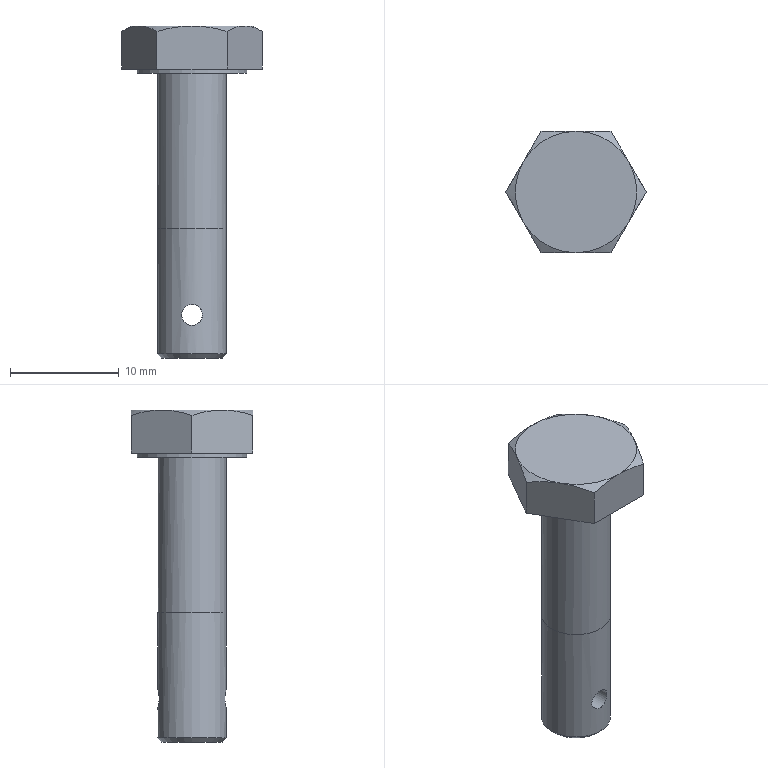Part | NX | features solid 2 | 1 solid | 21 faces | box 12.905 x 11.176 x 30.563 mm | volume 1269 mm3 | plane 10 | cone 7 | cylinder 4 | commonest cylinder face diameters 6.35 x2 1.93 x1 10.109 x1
STEP:
#1=CARTESIAN_POINT('',(0.,-3.175,-27.559));
#2=VERTEX_POINT('',#1);
#3=CARTESIAN_POINT('',(0.7569,-3.102,-27.35));
#4=CARTESIAN_POINT('',(-0.00006064,-3.212,-27.664));
#5=CARTESIAN_POINT('',(-0.7566,-3.102,-27.349));
#6=CARTESIAN_POINT('',(-1.07,-2.986,-26.595));
#7=CARTESIAN_POINT('',(-0.7562,-3.102,-25.837));
#8=CARTESIAN_POINT('',(-0.0005897,-3.212,-25.524));
#9=CARTESIAN_POINT('',(0.7561,-3.102,-25.837));
#10=CARTESIAN_POINT('',(1.07,-2.986,-26.594));
#11=CARTESIAN_POINT('',(0.7569,-3.102,-27.35));
#12=CARTESIAN_POINT('',(-0.00006064,-3.212,-27.664));
#13=CARTESIAN_POINT('',(-0.7566,-3.102,-27.349));
#14=B_SPLINE_CURVE_WITH_KNOTS('',3,(#3,#4,#5,#6,#7,#8,#9,#10,#11,#12,#13),.UNSPECIFIED.,.T.,.F.,(1,1,1,1,1,1,1,1,1,1,1,1,1,1,1),(-0.002276,-0.001518,-0.0007588,0.,0.0007588,0.001518,0.002276,0.003035,0.003794,0.004553,0.005312,0.006071,0.006829,0.007588,0.008347),.UNSPECIFIED.);
#15=EDGE_CURVE('',#2,#2,#14,.T.);
#16=ORIENTED_EDGE('',*,*,#15,.T.);
#17=EDGE_LOOP('',(#16));
#18=FACE_BOUND('',#17,.T.);
#19=CARTESIAN_POINT('',(-3.175,0.,-18.656));
#20=VERTEX_POINT('',#19);
#21=CARTESIAN_POINT('',(-2.488,2.488,-18.656));
#22=CARTESIAN_POINT('',(-3.519,0.,-18.656));
#23=CARTESIAN_POINT('',(-2.488,-2.488,-18.656));
#24=CARTESIAN_POINT('',(0.,-3.519,-18.656));
#25=CARTESIAN_POINT('',(2.488,-2.488,-18.656));
#26=CARTESIAN_POINT('',(3.519,0.,-18.656));
#27=CARTESIAN_POINT('',(2.488,2.488,-18.656));
#28=CARTESIAN_POINT('',(0.,3.519,-18.656));
#29=CARTESIAN_POINT('',(-2.488,2.488,-18.656));
#30=CARTESIAN_POINT('',(-3.519,0.,-18.656));
#31=CARTESIAN_POINT('',(-2.488,-2.488,-18.656));
#32=B_SPLINE_CURVE_WITH_KNOTS('',3,(#21,#22,#23,#24,#25,#26,#27,#28,#29,#30,#31),.UNSPECIFIED.,.T.,.F.,(1,1,1,1,1,1,1,1,1,1,1,1,1,1,1),(-0.375,-0.25,-0.125,0.,0.125,0.25,0.375,0.5,0.625,0.75,0.875,1.,1.125,1.25,1.375),.UNSPECIFIED.);
#33=EDGE_CURVE('',#20,#20,#32,.T.);
#34=ORIENTED_EDGE('',*,*,#33,.F.);
#35=EDGE_LOOP('',(#34));
#36=FACE_BOUND('',#35,.T.);
#37=CARTESIAN_POINT('',(-3.175,0.,-30.182));
#38=VERTEX_POINT('',#37);
#39=CARTESIAN_POINT('',(0.,0.,-30.182));
#40=DIRECTION('',(0.,0.,-1.));
#41=DIRECTION('',(-1.,0.,0.));
#42=AXIS2_PLACEMENT_3D('',#39,#40,#41);
#43=CIRCLE('',#42,3.175);
#44=EDGE_CURVE('',#38,#38,#43,.T.);
#45=ORIENTED_EDGE('',*,*,#44,.F.);
#46=EDGE_LOOP('',(#45));
#47=FACE_BOUND('',#46,.T.);
#48=CARTESIAN_POINT('',(0.,3.175,-27.559));
#49=VERTEX_POINT('',#48);
#50=CARTESIAN_POINT('',(-0.7569,3.102,-27.35));
#51=CARTESIAN_POINT('',(0.00006064,3.212,-27.664));
#52=CARTESIAN_POINT('',(0.7566,3.102,-27.349));
#53=CARTESIAN_POINT('',(1.07,2.986,-26.595));
#54=CARTESIAN_POINT('',(0.7562,3.102,-25.837));
#55=CARTESIAN_POINT('',(0.0005897,3.212,-25.524));
#56=CARTESIAN_POINT('',(-0.7561,3.102,-25.837));
#57=CARTESIAN_POINT('',(-1.07,2.986,-26.594));
#58=CARTESIAN_POINT('',(-0.7569,3.102,-27.35));
#59=CARTESIAN_POINT('',(0.00006064,3.212,-27.664));
#60=CARTESIAN_POINT('',(0.7566,3.102,-27.349));
#61=B_SPLINE_CURVE_WITH_KNOTS('',3,(#50,#51,#52,#53,#54,#55,#56,#57,#58,#59,#60),.UNSPECIFIED.,.T.,.F.,(1,1,1,1,1,1,1,1,1,1,1,1,1,1,1),(-0.002276,-0.001518,-0.0007588,0.,0.0007588,0.001518,0.002276,0.003035,0.003794,0.004553,0.005312,0.006071,0.006829,0.007588,0.008347),.UNSPECIFIED.);
#62=EDGE_CURVE('',#49,#49,#61,.T.);
#63=ORIENTED_EDGE('',*,*,#62,.T.);
#64=EDGE_LOOP('',(#63));
#65=FACE_BOUND('',#64,.T.);
#66=CARTESIAN_POINT('',(0.,0.,0.));
#67=DIRECTION('',(0.,0.,-1.));
#68=DIRECTION('',(-1.,0.,0.));
#69=AXIS2_PLACEMENT_3D('',#66,#67,#68);
#70=CYLINDRICAL_SURFACE('',#69,3.175);
#71=ADVANCED_FACE('',(#18,#36,#47,#65),#70,.T.);
#72=CARTESIAN_POINT('',(-3.175,0.,-4.369));
#73=VERTEX_POINT('',#72);
#74=CARTESIAN_POINT('',(0.,0.,-4.369));
#75=DIRECTION('',(0.,0.,-1.));
#76=DIRECTION('',(-1.,0.,0.));
#77=AXIS2_PLACEMENT_3D('',#74,#75,#76);
#78=CIRCLE('',#77,3.175);
#79=EDGE_CURVE('',#73,#73,#78,.T.);
#80=ORIENTED_EDGE('',*,*,#79,.T.);
#81=EDGE_LOOP('',(#80));
#82=FACE_BOUND('',#81,.T.);
#83=ORIENTED_EDGE('',*,*,#33,.T.);
#84=EDGE_LOOP('',(#83));
#85=FACE_BOUND('',#84,.T.);
#86=CARTESIAN_POINT('',(0.,0.,0.));
#87=DIRECTION('',(0.,0.,-1.));
#88=DIRECTION('',(-1.,0.,0.));
#89=AXIS2_PLACEMENT_3D('',#86,#87,#88);
#90=CYLINDRICAL_SURFACE('',#89,3.175);
#91=ADVANCED_FACE('',(#82,#85),#90,.T.);
#92=CARTESIAN_POINT('',(-6.452,0.,-3.962));
#93=VERTEX_POINT('',#92);
#94=CARTESIAN_POINT('',(-3.226,5.588,-3.962));
#95=VERTEX_POINT('',#94);
#96=CARTESIAN_POINT('',(-3.576,4.983,-3.962));
#97=DIRECTION('',(0.5,0.866,0.));
#98=VECTOR('',#97,1000.);
#99=LINE('',#96,#98);
#100=EDGE_CURVE('',#93,#95,#99,.T.);
#101=ORIENTED_EDGE('',*,*,#100,.T.);
#102=CARTESIAN_POINT('',(3.226,5.588,-3.962));
#103=VERTEX_POINT('',#102);
#104=CARTESIAN_POINT('',(5.055,5.588,-3.962));
#105=DIRECTION('',(1.,0.,0.));
#106=VECTOR('',#105,1000.);
#107=LINE('',#104,#106);
#108=EDGE_CURVE('',#95,#103,#107,.T.);
#109=ORIENTED_EDGE('',*,*,#108,.T.);
#110=CARTESIAN_POINT('',(6.452,0.,-3.962));
#111=VERTEX_POINT('',#110);
#112=CARTESIAN_POINT('',(6.103,0.6053,-3.962));
#113=DIRECTION('',(0.5,-0.866,0.));
#114=VECTOR('',#113,1000.);
#115=LINE('',#112,#114);
#116=EDGE_CURVE('',#103,#111,#115,.T.);
#117=ORIENTED_EDGE('',*,*,#116,.T.);
#118=CARTESIAN_POINT('',(3.226,-5.588,-3.962));
#119=VERTEX_POINT('',#118);
#120=CARTESIAN_POINT('',(6.103,-0.6053,-3.962));
#121=DIRECTION('',(-0.5,-0.866,0.));
#122=VECTOR('',#121,1000.);
#123=LINE('',#120,#122);
#124=EDGE_CURVE('',#111,#119,#123,.T.);
#125=ORIENTED_EDGE('',*,*,#124,.T.);
#126=CARTESIAN_POINT('',(-3.226,-5.588,-3.962));
#127=VERTEX_POINT('',#126);
#128=CARTESIAN_POINT('',(5.055,-5.588,-3.962));
#129=DIRECTION('',(-1.,0.,0.));
#130=VECTOR('',#129,1000.);
#131=LINE('',#128,#130);
#132=EDGE_CURVE('',#119,#127,#131,.T.);
#133=ORIENTED_EDGE('',*,*,#132,.T.);
#134=CARTESIAN_POINT('',(-3.576,-4.983,-3.962));
#135=DIRECTION('',(-0.5,0.866,0.));
#136=VECTOR('',#135,1000.);
#137=LINE('',#134,#136);
#138=EDGE_CURVE('',#127,#93,#137,.T.);
#139=ORIENTED_EDGE('',*,*,#138,.T.);
#140=EDGE_LOOP('',(#101,#109,#117,#125,#133,#139));
#141=FACE_BOUND('',#140,.T.);
#142=CARTESIAN_POINT('',(-5.055,0.,-3.962));
#143=VERTEX_POINT('',#142);
#144=CARTESIAN_POINT('',(0.,0.,-3.962));
#145=DIRECTION('',(0.,0.,-1.));
#146=DIRECTION('',(-1.,0.,0.));
#147=AXIS2_PLACEMENT_3D('',#144,#145,#146);
#148=CIRCLE('',#147,5.055);
#149=EDGE_CURVE('',#143,#143,#148,.T.);
#150=ORIENTED_EDGE('',*,*,#149,.F.);
#151=EDGE_LOOP('',(#150));
#152=FACE_BOUND('',#151,.T.);
#153=CARTESIAN_POINT('',(5.055,0.,-3.962));
#154=DIRECTION('',(0.,0.,-1.));
#155=DIRECTION('',(-1.,0.,0.));
#156=AXIS2_PLACEMENT_3D('',#153,#154,#155);
#157=PLANE('',#156);
#158=ADVANCED_FACE('',(#141,#152),#157,.T.);
#159=CARTESIAN_POINT('',(-2.794,0.,-30.563));
#160=VERTEX_POINT('',#159);
#161=CARTESIAN_POINT('',(0.,0.,-30.563));
#162=DIRECTION('',(0.,0.,-1.));
#163=DIRECTION('',(-1.,0.,0.));
#164=AXIS2_PLACEMENT_3D('',#161,#162,#163);
#165=CIRCLE('',#164,2.794);
#166=EDGE_CURVE('',#160,#160,#165,.T.);
#167=ORIENTED_EDGE('',*,*,#166,.T.);
#168=EDGE_LOOP('',(#167));
#169=FACE_BOUND('',#168,.T.);
#170=CARTESIAN_POINT('',(0.,0.,-30.563));
#171=DIRECTION('',(0.,0.,-1.));
#172=DIRECTION('',(-1.,0.,0.));
#173=AXIS2_PLACEMENT_3D('',#170,#171,#172);
#174=PLANE('',#173);
#175=ADVANCED_FACE('',(#169),#174,.T.);
#176=ORIENTED_EDGE('',*,*,#44,.T.);
#177=EDGE_LOOP('',(#176));
#178=FACE_BOUND('',#177,.T.);
#179=ORIENTED_EDGE('',*,*,#166,.F.);
#180=EDGE_LOOP('',(#179));
#181=FACE_BOUND('',#180,.T.);
#182=CARTESIAN_POINT('',(0.,0.,-30.563));
#183=DIRECTION('',(0.,0.,1.));
#184=DIRECTION('',(1.,0.,0.));
#185=AXIS2_PLACEMENT_3D('',#182,#183,#184);
#186=CONICAL_SURFACE('',#185,2.794,0.7854);
#187=ADVANCED_FACE('',(#178,#181),#186,.T.);
#188=CARTESIAN_POINT('',(-5.055,0.,-4.369));
#189=VERTEX_POINT('',#188);
#190=CARTESIAN_POINT('',(0.,0.,-4.369));
#191=DIRECTION('',(0.,0.,-1.));
#192=DIRECTION('',(-1.,0.,0.));
#193=AXIS2_PLACEMENT_3D('',#190,#191,#192);
#194=CIRCLE('',#193,5.055);
#195=EDGE_CURVE('',#189,#189,#194,.T.);
#196=ORIENTED_EDGE('',*,*,#195,.T.);
#197=EDGE_LOOP('',(#196));
#198=FACE_BOUND('',#197,.T.);
#199=ORIENTED_EDGE('',*,*,#79,.F.);
#200=EDGE_LOOP('',(#199));
#201=FACE_BOUND('',#200,.T.);
#202=CARTESIAN_POINT('',(3.175,0.,-4.369));
#203=DIRECTION('',(0.,0.,-1.));
#204=DIRECTION('',(-1.,0.,0.));
#205=AXIS2_PLACEMENT_3D('',#202,#203,#204);
#206=PLANE('',#205);
#207=ADVANCED_FACE('',(#198,#201),#206,.T.);
#208=ORIENTED_EDGE('',*,*,#149,.T.);
#209=EDGE_LOOP('',(#208));
#210=FACE_BOUND('',#209,.T.);
#211=ORIENTED_EDGE('',*,*,#195,.F.);
#212=EDGE_LOOP('',(#211));
#213=FACE_BOUND('',#212,.T.);
#214=CARTESIAN_POINT('',(0.,0.,0.));
#215=DIRECTION('',(0.,0.,-1.));
#216=DIRECTION('',(-1.,0.,0.));
#217=AXIS2_PLACEMENT_3D('',#214,#215,#216);
#218=CYLINDRICAL_SURFACE('',#217,5.055);
#219=ADVANCED_FACE('',(#210,#213),#218,.T.);
#220=ORIENTED_EDGE('',*,*,#108,.F.);
#221=CARTESIAN_POINT('',(-3.226,5.588,-0.4991));
#222=VERTEX_POINT('',#221);
#223=CARTESIAN_POINT('',(-3.226,5.588,-33.619));
#224=DIRECTION('',(0.,0.,1.));
#225=VECTOR('',#224,1000.);
#226=LINE('',#223,#225);
#227=EDGE_CURVE('',#95,#222,#226,.T.);
#228=ORIENTED_EDGE('',*,*,#227,.T.);
#229=CARTESIAN_POINT('',(0.,5.588,0.));
#230=VERTEX_POINT('',#229);
#231=CARTESIAN_POINT('',(-3.226,5.588,-0.4991));
#232=CARTESIAN_POINT('',(-2.177,5.588,-0.1961));
#233=CARTESIAN_POINT('',(-1.09,5.588,0.));
#234=CARTESIAN_POINT('',(0.,5.588,0.));
#235=B_SPLINE_CURVE_WITH_KNOTS('',3,(#231,#232,#233,#234),.UNSPECIFIED.,.F.,.F.,(4,4),(0.005758,0.009022),.UNSPECIFIED.);
#236=EDGE_CURVE('',#230,#222,#235,.F.);
#237=ORIENTED_EDGE('',*,*,#236,.F.);
#238=CARTESIAN_POINT('',(3.226,5.588,-0.4991));
#239=VERTEX_POINT('',#238);
#240=CARTESIAN_POINT('',(0.,5.588,0.));
#241=CARTESIAN_POINT('',(1.091,5.588,0.));
#242=CARTESIAN_POINT('',(2.183,5.588,-0.1979));
#243=CARTESIAN_POINT('',(3.226,5.588,-0.4991));
#244=B_SPLINE_CURVE_WITH_KNOTS('',3,(#240,#241,#242,#243),.UNSPECIFIED.,.F.,.F.,(4,4),(0.009022,0.01229),.UNSPECIFIED.);
#245=EDGE_CURVE('',#239,#230,#244,.F.);
#246=ORIENTED_EDGE('',*,*,#245,.F.);
#247=CARTESIAN_POINT('',(3.226,5.588,-33.619));
#248=DIRECTION('',(0.,0.,1.));
#249=VECTOR('',#248,1000.);
#250=LINE('',#247,#249);
#251=EDGE_CURVE('',#103,#239,#250,.T.);
#252=ORIENTED_EDGE('',*,*,#251,.F.);
#253=EDGE_LOOP('',(#220,#228,#237,#246,#252));
#254=FACE_BOUND('',#253,.T.);
#255=CARTESIAN_POINT('',(3.226,5.588,-33.619));
#256=DIRECTION('',(0.,1.,0.));
#257=DIRECTION('',(0.,0.,1.));
#258=AXIS2_PLACEMENT_3D('',#255,#256,#257);
#259=PLANE('',#258);
#260=ADVANCED_FACE('',(#254),#259,.T.);
#261=ORIENTED_EDGE('',*,*,#100,.F.);
#262=CARTESIAN_POINT('',(-6.452,0.,-0.4991));
#263=VERTEX_POINT('',#262);
#264=CARTESIAN_POINT('',(-6.452,0.,-33.619));
#265=DIRECTION('',(0.,0.,1.));
#266=VECTOR('',#265,1000.);
#267=LINE('',#264,#266);
#268=EDGE_CURVE('',#93,#263,#267,.T.);
#269=ORIENTED_EDGE('',*,*,#268,.T.);
#270=CARTESIAN_POINT('',(-4.839,2.794,0.));
#271=VERTEX_POINT('',#270);
#272=CARTESIAN_POINT('',(-4.839,2.794,0.));
#273=CARTESIAN_POINT('',(-5.387,1.846,0.));
#274=CARTESIAN_POINT('',(-5.926,0.9118,-0.1952));
#275=CARTESIAN_POINT('',(-6.452,0.,-0.4991));
#276=B_SPLINE_CURVE_WITH_KNOTS('',3,(#272,#273,#274,#275),.UNSPECIFIED.,.F.,.F.,(4,4),(0.003265,0.006517),.UNSPECIFIED.);
#277=EDGE_CURVE('',#271,#263,#276,.T.);
#278=ORIENTED_EDGE('',*,*,#277,.F.);
#279=CARTESIAN_POINT('',(-3.226,5.588,-0.4991));
#280=CARTESIAN_POINT('',(-3.754,4.674,-0.1944));
#281=CARTESIAN_POINT('',(-4.29,3.746,0.));
#282=CARTESIAN_POINT('',(-4.839,2.794,0.));
#283=B_SPLINE_CURVE_WITH_KNOTS('',3,(#279,#280,#281,#282),.UNSPECIFIED.,.F.,.F.,(4,4),(0.000000238,0.003265),.UNSPECIFIED.);
#284=EDGE_CURVE('',#222,#271,#283,.T.);
#285=ORIENTED_EDGE('',*,*,#284,.F.);
#286=ORIENTED_EDGE('',*,*,#227,.F.);
#287=EDGE_LOOP('',(#261,#269,#278,#285,#286));
#288=FACE_BOUND('',#287,.T.);
#289=CARTESIAN_POINT('',(-3.226,5.588,-33.619));
#290=DIRECTION('',(-0.866,0.5,0.));
#291=DIRECTION('',(-0.5,-0.866,0.));
#292=AXIS2_PLACEMENT_3D('',#289,#290,#291);
#293=PLANE('',#292);
#294=ADVANCED_FACE('',(#288),#293,.T.);
#295=ORIENTED_EDGE('',*,*,#138,.F.);
#296=CARTESIAN_POINT('',(-3.226,-5.588,-0.4991));
#297=VERTEX_POINT('',#296);
#298=CARTESIAN_POINT('',(-3.226,-5.588,-33.619));
#299=DIRECTION('',(0.,0.,1.));
#300=VECTOR('',#299,1000.);
#301=LINE('',#298,#300);
#302=EDGE_CURVE('',#127,#297,#301,.T.);
#303=ORIENTED_EDGE('',*,*,#302,.T.);
#304=CARTESIAN_POINT('',(-4.839,-2.794,0.));
#305=VERTEX_POINT('',#304);
#306=CARTESIAN_POINT('',(-4.839,-2.794,0.));
#307=CARTESIAN_POINT('',(-4.292,-3.742,0.));
#308=CARTESIAN_POINT('',(-3.753,-4.676,-0.1952));
#309=CARTESIAN_POINT('',(-3.226,-5.588,-0.4991));
#310=B_SPLINE_CURVE_WITH_KNOTS('',3,(#306,#307,#308,#309),.UNSPECIFIED.,.F.,.F.,(4,4),(0.003265,0.006517),.UNSPECIFIED.);
#311=EDGE_CURVE('',#305,#297,#310,.T.);
#312=ORIENTED_EDGE('',*,*,#311,.F.);
#313=CARTESIAN_POINT('',(-6.452,0.,-0.4991));
#314=CARTESIAN_POINT('',(-5.925,-0.9141,-0.1944));
#315=CARTESIAN_POINT('',(-5.389,-1.842,0.));
#316=CARTESIAN_POINT('',(-4.839,-2.794,0.));
#317=B_SPLINE_CURVE_WITH_KNOTS('',3,(#313,#314,#315,#316),.UNSPECIFIED.,.F.,.F.,(4,4),(0.000000238,0.003265),.UNSPECIFIED.);
#318=EDGE_CURVE('',#263,#305,#317,.T.);
#319=ORIENTED_EDGE('',*,*,#318,.F.);
#320=ORIENTED_EDGE('',*,*,#268,.F.);
#321=EDGE_LOOP('',(#295,#303,#312,#319,#320));
#322=FACE_BOUND('',#321,.T.);
#323=CARTESIAN_POINT('',(-6.452,0.,-33.619));
#324=DIRECTION('',(-0.866,-0.5,0.));
#325=DIRECTION('',(0.5,-0.866,0.));
#326=AXIS2_PLACEMENT_3D('',#323,#324,#325);
#327=PLANE('',#326);
#328=ADVANCED_FACE('',(#322),#327,.T.);
#329=ORIENTED_EDGE('',*,*,#132,.F.);
#330=CARTESIAN_POINT('',(3.226,-5.588,-0.4991));
#331=VERTEX_POINT('',#330);
#332=CARTESIAN_POINT('',(3.226,-5.588,-33.619));
#333=DIRECTION('',(0.,0.,1.));
#334=VECTOR('',#333,1000.);
#335=LINE('',#332,#334);
#336=EDGE_CURVE('',#119,#331,#335,.T.);
#337=ORIENTED_EDGE('',*,*,#336,.T.);
#338=CARTESIAN_POINT('',(0.,-5.588,0.));
#339=VERTEX_POINT('',#338);
#340=CARTESIAN_POINT('',(0.,-5.588,0.));
#341=CARTESIAN_POINT('',(1.091,-5.588,0.));
#342=CARTESIAN_POINT('',(2.183,-5.588,-0.1979));
#343=CARTESIAN_POINT('',(3.226,-5.588,-0.4991));
#344=B_SPLINE_CURVE_WITH_KNOTS('',3,(#340,#341,#342,#343),.UNSPECIFIED.,.F.,.F.,(4,4),(0.009022,0.01229),.UNSPECIFIED.);
#345=EDGE_CURVE('',#339,#331,#344,.T.);
#346=ORIENTED_EDGE('',*,*,#345,.F.);
#347=CARTESIAN_POINT('',(-3.226,-5.588,-0.4991));
#348=CARTESIAN_POINT('',(-2.177,-5.588,-0.1961));
#349=CARTESIAN_POINT('',(-1.09,-5.588,0.));
#350=CARTESIAN_POINT('',(0.,-5.588,0.));
#351=B_SPLINE_CURVE_WITH_KNOTS('',3,(#347,#348,#349,#350),.UNSPECIFIED.,.F.,.F.,(4,4),(0.005758,0.009022),.UNSPECIFIED.);
#352=EDGE_CURVE('',#297,#339,#351,.T.);
#353=ORIENTED_EDGE('',*,*,#352,.F.);
#354=ORIENTED_EDGE('',*,*,#302,.F.);
#355=EDGE_LOOP('',(#329,#337,#346,#353,#354));
#356=FACE_BOUND('',#355,.T.);
#357=CARTESIAN_POINT('',(-3.226,-5.588,-33.619));
#358=DIRECTION('',(0.,-1.,0.));
#359=DIRECTION('',(0.,0.,-1.));
#360=AXIS2_PLACEMENT_3D('',#357,#358,#359);
#361=PLANE('',#360);
#362=ADVANCED_FACE('',(#356),#361,.T.);
#363=ORIENTED_EDGE('',*,*,#124,.F.);
#364=CARTESIAN_POINT('',(6.452,0.,-0.4991));
#365=VERTEX_POINT('',#364);
#366=CARTESIAN_POINT('',(6.452,0.,-33.619));
#367=DIRECTION('',(0.,0.,1.));
#368=VECTOR('',#367,1000.);
#369=LINE('',#366,#368);
#370=EDGE_CURVE('',#111,#365,#369,.T.);
#371=ORIENTED_EDGE('',*,*,#370,.T.);
#372=CARTESIAN_POINT('',(4.839,-2.794,0.));
#373=VERTEX_POINT('',#372);
#374=CARTESIAN_POINT('',(4.839,-2.794,0.));
#375=CARTESIAN_POINT('',(5.387,-1.846,0.));
#376=CARTESIAN_POINT('',(5.926,-0.9118,-0.1952));
#377=CARTESIAN_POINT('',(6.452,0.,-0.4991));
#378=B_SPLINE_CURVE_WITH_KNOTS('',3,(#374,#375,#376,#377),.UNSPECIFIED.,.F.,.F.,(4,4),(0.003265,0.006517),.UNSPECIFIED.);
#379=EDGE_CURVE('',#373,#365,#378,.T.);
#380=ORIENTED_EDGE('',*,*,#379,.F.);
#381=CARTESIAN_POINT('',(3.226,-5.588,-0.4991));
#382=CARTESIAN_POINT('',(3.754,-4.674,-0.1944));
#383=CARTESIAN_POINT('',(4.29,-3.746,0.));
#384=CARTESIAN_POINT('',(4.839,-2.794,0.));
#385=B_SPLINE_CURVE_WITH_KNOTS('',3,(#381,#382,#383,#384),.UNSPECIFIED.,.F.,.F.,(4,4),(0.000000238,0.003265),.UNSPECIFIED.);
#386=EDGE_CURVE('',#331,#373,#385,.T.);
#387=ORIENTED_EDGE('',*,*,#386,.F.);
#388=ORIENTED_EDGE('',*,*,#336,.F.);
#389=EDGE_LOOP('',(#363,#371,#380,#387,#388));
#390=FACE_BOUND('',#389,.T.);
#391=CARTESIAN_POINT('',(3.226,-5.588,-33.619));
#392=DIRECTION('',(0.866,-0.5,0.));
#393=DIRECTION('',(0.5,0.866,0.));
#394=AXIS2_PLACEMENT_3D('',#391,#392,#393);
#395=PLANE('',#394);
#396=ADVANCED_FACE('',(#390),#395,.T.);
#397=ORIENTED_EDGE('',*,*,#116,.F.);
#398=ORIENTED_EDGE('',*,*,#251,.T.);
#399=CARTESIAN_POINT('',(4.839,2.794,0.));
#400=VERTEX_POINT('',#399);
#401=CARTESIAN_POINT('',(4.839,2.794,0.));
#402=CARTESIAN_POINT('',(4.292,3.742,0.));
#403=CARTESIAN_POINT('',(3.753,4.676,-0.1952));
#404=CARTESIAN_POINT('',(3.226,5.588,-0.4991));
#405=B_SPLINE_CURVE_WITH_KNOTS('',3,(#401,#402,#403,#404),.UNSPECIFIED.,.F.,.F.,(4,4),(0.003265,0.006517),.UNSPECIFIED.);
#406=EDGE_CURVE('',#400,#239,#405,.T.);
#407=ORIENTED_EDGE('',*,*,#406,.F.);
#408=CARTESIAN_POINT('',(6.452,0.,-0.4991));
#409=CARTESIAN_POINT('',(5.925,0.9141,-0.1944));
#410=CARTESIAN_POINT('',(5.389,1.842,0.));
#411=CARTESIAN_POINT('',(4.839,2.794,0.));
#412=B_SPLINE_CURVE_WITH_KNOTS('',3,(#408,#409,#410,#411),.UNSPECIFIED.,.F.,.F.,(4,4),(0.000000238,0.003265),.UNSPECIFIED.);
#413=EDGE_CURVE('',#365,#400,#412,.T.);
#414=ORIENTED_EDGE('',*,*,#413,.F.);
#415=ORIENTED_EDGE('',*,*,#370,.F.);
#416=EDGE_LOOP('',(#397,#398,#407,#414,#415));
#417=FACE_BOUND('',#416,.T.);
#418=CARTESIAN_POINT('',(6.452,0.,-33.619));
#419=DIRECTION('',(0.866,0.5,0.));
#420=DIRECTION('',(-0.5,0.866,0.));
#421=AXIS2_PLACEMENT_3D('',#418,#419,#420);
#422=PLANE('',#421);
#423=ADVANCED_FACE('',(#417),#422,.T.);
#424=CARTESIAN_POINT('',(0.,0.,0.));
#425=DIRECTION('',(0.,0.,-1.));
#426=DIRECTION('',(-1.,0.,0.));
#427=AXIS2_PLACEMENT_3D('',#424,#425,#426);
#428=CIRCLE('',#427,5.588);
#429=EDGE_CURVE('',#400,#373,#428,.T.);
#430=ORIENTED_EDGE('',*,*,#429,.T.);
#431=ORIENTED_EDGE('',*,*,#379,.T.);
#432=ORIENTED_EDGE('',*,*,#413,.T.);
#433=EDGE_LOOP('',(#430,#431,#432));
#434=FACE_BOUND('',#433,.T.);
#435=CARTESIAN_POINT('',(0.,0.,-0.5133));
#436=DIRECTION('',(0.,0.,-1.));
#437=DIRECTION('',(-1.,0.,0.));
#438=AXIS2_PLACEMENT_3D('',#435,#436,#437);
#439=CONICAL_SURFACE('',#438,6.477,1.047);
#440=ADVANCED_FACE('',(#434),#439,.T.);
#441=CARTESIAN_POINT('',(0.,0.,0.));
#442=DIRECTION('',(0.,0.,-1.));
#443=DIRECTION('',(-1.,0.,0.));
#444=AXIS2_PLACEMENT_3D('',#441,#442,#443);
#445=CIRCLE('',#444,5.588);
#446=EDGE_CURVE('',#373,#339,#445,.T.);
#447=ORIENTED_EDGE('',*,*,#446,.T.);
#448=ORIENTED_EDGE('',*,*,#345,.T.);
#449=ORIENTED_EDGE('',*,*,#386,.T.);
#450=EDGE_LOOP('',(#447,#448,#449));
#451=FACE_BOUND('',#450,.T.);
#452=CARTESIAN_POINT('',(0.,0.,-0.5133));
#453=DIRECTION('',(0.,0.,-1.));
#454=DIRECTION('',(-1.,0.,0.));
#455=AXIS2_PLACEMENT_3D('',#452,#453,#454);
#456=CONICAL_SURFACE('',#455,6.477,1.047);
#457=ADVANCED_FACE('',(#451),#456,.T.);
#458=CARTESIAN_POINT('',(0.,0.,0.));
#459=DIRECTION('',(0.,0.,-1.));
#460=DIRECTION('',(-1.,0.,0.));
#461=AXIS2_PLACEMENT_3D('',#458,#459,#460);
#462=CIRCLE('',#461,5.588);
#463=EDGE_CURVE('',#339,#305,#462,.T.);
#464=ORIENTED_EDGE('',*,*,#463,.T.);
#465=ORIENTED_EDGE('',*,*,#311,.T.);
#466=ORIENTED_EDGE('',*,*,#352,.T.);
#467=EDGE_LOOP('',(#464,#465,#466));
#468=FACE_BOUND('',#467,.T.);
#469=CARTESIAN_POINT('',(0.,0.,-0.5133));
#470=DIRECTION('',(0.,0.,-1.));
#471=DIRECTION('',(-1.,0.,0.));
#472=AXIS2_PLACEMENT_3D('',#469,#470,#471);
#473=CONICAL_SURFACE('',#472,6.477,1.047);
#474=ADVANCED_FACE('',(#468),#473,.T.);
#475=CARTESIAN_POINT('',(0.,0.,0.));
#476=DIRECTION('',(0.,0.,-1.));
#477=DIRECTION('',(-1.,0.,0.));
#478=AXIS2_PLACEMENT_3D('',#475,#476,#477);
#479=CIRCLE('',#478,5.588);
#480=EDGE_CURVE('',#305,#271,#479,.T.);
#481=ORIENTED_EDGE('',*,*,#480,.T.);
#482=ORIENTED_EDGE('',*,*,#277,.T.);
#483=ORIENTED_EDGE('',*,*,#318,.T.);
#484=EDGE_LOOP('',(#481,#482,#483));
#485=FACE_BOUND('',#484,.T.);
#486=CARTESIAN_POINT('',(0.,0.,-0.5133));
#487=DIRECTION('',(0.,0.,-1.));
#488=DIRECTION('',(-1.,0.,0.));
#489=AXIS2_PLACEMENT_3D('',#486,#487,#488);
#490=CONICAL_SURFACE('',#489,6.477,1.047);
#491=ADVANCED_FACE('',(#485),#490,.T.);
#492=CARTESIAN_POINT('',(0.,0.,0.));
#493=DIRECTION('',(0.,0.,-1.));
#494=DIRECTION('',(-1.,0.,0.));
#495=AXIS2_PLACEMENT_3D('',#492,#493,#494);
#496=CIRCLE('',#495,5.588);
#497=EDGE_CURVE('',#271,#230,#496,.T.);
#498=ORIENTED_EDGE('',*,*,#497,.T.);
#499=ORIENTED_EDGE('',*,*,#236,.T.);
#500=ORIENTED_EDGE('',*,*,#284,.T.);
#501=EDGE_LOOP('',(#498,#499,#500));
#502=FACE_BOUND('',#501,.T.);
#503=CARTESIAN_POINT('',(0.,0.,-0.5133));
#504=DIRECTION('',(0.,0.,-1.));
#505=DIRECTION('',(-1.,0.,0.));
#506=AXIS2_PLACEMENT_3D('',#503,#504,#505);
#507=CONICAL_SURFACE('',#506,6.477,1.047);
#508=ADVANCED_FACE('',(#502),#507,.T.);
#509=ORIENTED_EDGE('',*,*,#497,.F.);
#510=ORIENTED_EDGE('',*,*,#480,.F.);
#511=ORIENTED_EDGE('',*,*,#463,.F.);
#512=ORIENTED_EDGE('',*,*,#446,.F.);
#513=ORIENTED_EDGE('',*,*,#429,.F.);
#514=CARTESIAN_POINT('',(0.,0.,0.));
#515=DIRECTION('',(0.,0.,-1.));
#516=DIRECTION('',(-1.,0.,0.));
#517=AXIS2_PLACEMENT_3D('',#514,#515,#516);
#518=CIRCLE('',#517,5.588);
#519=EDGE_CURVE('',#230,#400,#518,.T.);
#520=ORIENTED_EDGE('',*,*,#519,.F.);
#521=EDGE_LOOP('',(#509,#510,#511,#512,#513,#520));
#522=FACE_BOUND('',#521,.T.);
#523=CARTESIAN_POINT('',(5.588,0.,0.));
#524=DIRECTION('',(0.,0.,1.));
#525=DIRECTION('',(1.,0.,0.));
#526=AXIS2_PLACEMENT_3D('',#523,#524,#525);
#527=PLANE('',#526);
#528=ADVANCED_FACE('',(#522),#527,.T.);
#529=ORIENTED_EDGE('',*,*,#406,.T.);
#530=ORIENTED_EDGE('',*,*,#245,.T.);
#531=ORIENTED_EDGE('',*,*,#519,.T.);
#532=EDGE_LOOP('',(#529,#530,#531));
#533=FACE_BOUND('',#532,.T.);
#534=CARTESIAN_POINT('',(0.,0.,-0.5133));
#535=DIRECTION('',(0.,0.,-1.));
#536=DIRECTION('',(-1.,0.,0.));
#537=AXIS2_PLACEMENT_3D('',#534,#535,#536);
#538=CONICAL_SURFACE('',#537,6.477,1.047);
#539=ADVANCED_FACE('',(#533),#538,.T.);
#540=ORIENTED_EDGE('',*,*,#62,.F.);
#541=EDGE_LOOP('',(#540));
#542=FACE_BOUND('',#541,.T.);
#543=ORIENTED_EDGE('',*,*,#15,.F.);
#544=EDGE_LOOP('',(#543));
#545=FACE_BOUND('',#544,.T.);
#546=CARTESIAN_POINT('',(0.,6.147,-26.594));
#547=DIRECTION('',(0.,-1.,0.));
#548=DIRECTION('',(0.,0.,-1.));
#549=AXIS2_PLACEMENT_3D('',#546,#547,#548);
#550=CYLINDRICAL_SURFACE('',#549,0.9652);
#551=ADVANCED_FACE('',(#542,#545),#550,.F.);
#552=CLOSED_SHELL('',(#71,#91,#158,#175,#187,#207,#219,#260,#294,#328,#362,#396,#423,#440,#457,#474,#491,#508,#528,#539,#551));
#553=MANIFOLD_SOLID_BREP('',#552);
#554=(LENGTH_UNIT()NAMED_UNIT(*)SI_UNIT(.MILLI.,.METRE.));
#555=UNCERTAINTY_MEASURE_WITH_UNIT(LENGTH_MEASURE(0.0508),#554,'','');
#556=(NAMED_UNIT(*)PLANE_ANGLE_UNIT()SI_UNIT($,.RADIAN.));
#557=(NAMED_UNIT(*)SI_UNIT($,.STERADIAN.)SOLID_ANGLE_UNIT());
#558=(GEOMETRIC_REPRESENTATION_CONTEXT(3)GLOBAL_UNCERTAINTY_ASSIGNED_CONTEXT((#555))GLOBAL_UNIT_ASSIGNED_CONTEXT((#554,#556,#557))REPRESENTATION_CONTEXT('',''));
#559=ADVANCED_BREP_SHAPE_REPRESENTATION('',(#553),#558);